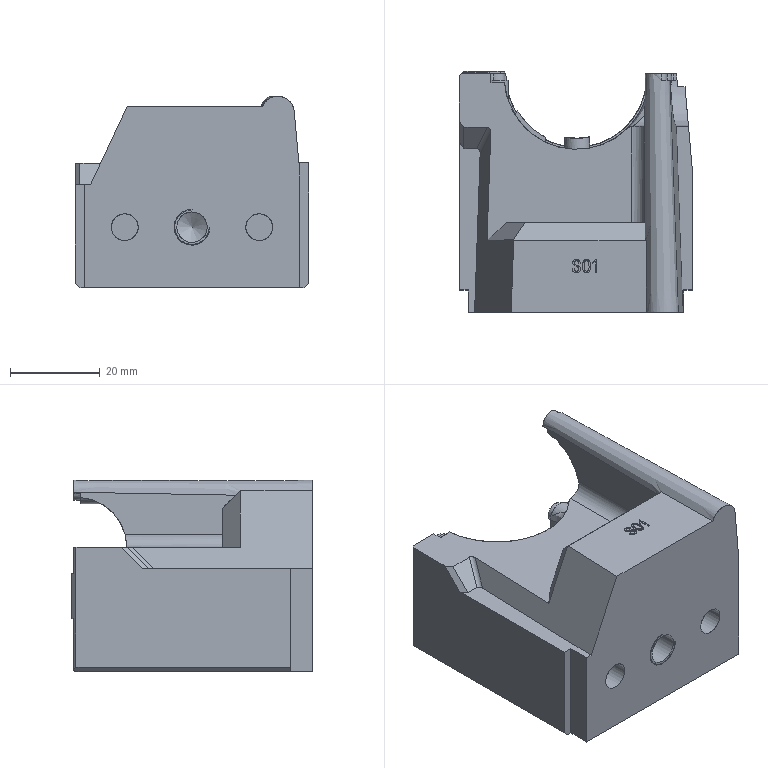NC program | PowerMill | posted with a generic post | part box 52 x 53.756 x 42.711 mm
Whole program:
%
O0001
N104 ( POWERMILL CB  : 2026004.0)
N105 ( POST VER      : 2026.0.0.5161)
N106 ( OPTION FILE   : FANUC)
N107 ( OUTPUT WORKPLANE : 2)
N108 (  )
N109 ( TOOL LIST )
N110 (--------------------------------)
N111 ( NO. | ID | DIA.| TIP RAD|LENGTH)
N112 (--------------------------------)
N113 (    1|D6_3| 6.0 |  0.0   | 97.0 )
N114 (--------------------------------)
N115 (  )
N116 ( NUMBER OF TOOLPATHS: 3.0 )
N117 ( ESTIMATED PROGRAM DURATION: 0 HOURS 1 MIN 8 SEC)
N118 (  )
N119 G00 G21 G80 G40 G17
N120 G90
N121 G54
N122 G53 Z0.0
N123 (---------------)
N124 ( START TOOLPATH : 13精光-D6-偏置平坦面 )
N125 (---------------)
N126 ( TOOL NO.    :1 )
N127 ( TOOL TYPE   : ENDMILL)
N128 ( TOOL ID     : D6_3)
N129 ( TOOL DIA    : 6.0 LENGTH 97.0)
N130 T1
N131 M6
N132 S6500 M03
N133 G00 G90 X-26.4454 Y-5.7682
N134 G43 Z75.756 H1
N135
N136 G05 P10000 R8
N137 Z53.3774
N138 G01 Z50.3774 F300.0
N139 X-24.9141 Y-2.9983 F500.0
N140 X-24.0418
N141 G02 X-25.9642 Y-0.039 I1.3749 J2.9971
N142 G01 X-25.9644 Y17.0037
N143 G02 X-23.7195 Y20.1236 I3.2977 J-0.0052
N144 G03 X-23.4367 Y20.3989 I-0.1638 J0.4512
N145 G00 Z61.2534
N146 G01 X-10.731 Y12.6007 F10000.0
N147 G00 Z56.2534
N148 G01 Z53.2534 F300.0
N149 X-13.5107 Y11.0873 F500.0
N150 X-19.0121 Y8.875
N151 G03 X-20.1113 Y8.6617 I-0.529 J-0.2127
N152 G01 X-20.1065 Y3.6989
N153 G03 X-19.4315 Y2.9984 I0.7017 J0.0007
N154 G01 X-19.1967 Y2.9895
N155 G03 X-18.4719 Y3.7613 I0.0266 J0.7012
N156 G01 X-18.9738 Y8.7197
N157 G03 X-19.0121 Y8.875 I-0.5675 J-0.0575
N158 G01 X-16.4541 Y9.9037
N159 X-16.8444 Y10.9904
N160 G02 X-16.9453 Y13.5394 I3.9938 J1.4346
N161 G01 X-16.8778 Y13.7875
N162 G03 X-21.8546 Y15.5141 I-2.5473 J0.6934
N163 G01 X-22.6473 Y13.6501
N164 G03 X-22.8609 Y12.6126 I2.4645 J-1.0481
N165 G01 X-22.9066 Y1.0939
N166 G03 X-21.6715 Y-0.1103 I1.2 J-0.0048
N167 G01 X-16.9207 Y0.0287
N168 G03 X-15.8315 Y0.8088 I-0.0351 J1.1995
N169 G01 X-15.7415 Y1.0503
N170 G03 X-15.6658 Y1.4681 I-1.1243 J0.4193
N171 G01 X-15.6593 Y6.3917
N172 G03 X-16.0952 Y8.9046 I-7.4049 J0.0097
N173 G01 X-16.4541 Y9.9037
N174 X-13.5107 Y11.0873
N175 G00 Z61.3534
N176 G01 X18.689 Y1.1883 F10000.0
N177 G00 Z56.3534
N178 G01 Z53.3534 F300.0
N179 X18.7509 Y1.2416 Z53.352
N180 X19.0519 Y1.6035 Z53.3437
N181 X19.2892 Y2.01 Z53.3355
N182 X19.4564 Y2.45 Z53.3273
N183 X19.5489 Y2.9115 Z53.3191
N184 X19.5642 Y3.382 Z53.3109
N185 X19.5018 Y3.8485 Z53.3027
N186 X19.3635 Y4.2985 Z53.2945
N187 X19.153 Y4.7195 Z53.2862
N188 X18.8761 Y5.1001 Z53.278
N189 X18.5403 Y5.43 Z53.2698
N190 X18.1548 Y5.7001 Z53.2616
N191 X17.7301 Y5.9031 Z53.2534
N192 X16.7998 Y6.2566 F500.0
N193 G03 X15.4447 Y5.4189 I-0.3565 J-0.9382
N194 G01 X15.1452 Y2.4429
N195 G03 X17.4406 Y-0.0864 I2.2876 J-0.2302
N196 G01 X24.7973 Y-0.0614
N197 G03 X25.7715 Y0.847 I-0.0033 J0.9801
N198 G01 X26.0144 Y4.1563
N199 G03 X24.5856 Y5.4215 I-1.1968 J0.0879
N200 G01 X24.2381 Y5.3531
N201 G02 X17.7301 Y5.9031 I-2.2935 J11.6409
N202 G01 X18.7117 Y8.4862
N203 G02 X16.7657 Y10.2425 I1.03 J3.0976
N204 G03 X16.3946 Y10.5136 I-0.4342 J-0.2047
N205 G02 X13.9637 Y11.6713 I0.5149 J4.2123
N206 G03 X13.3385 Y11.7026 I-0.3308 J-0.3478
N207 G01 X13.2771 Y11.6576
N208 G00 Z61.2534
N209 G01 X32.0704 Y11.1193 F10000.0
N210 G00 Z56.2534
N211 G01 Z53.2534 F300.0
N212 X28.9054 Y11.1194 F500.0
N213 G03 X28.7048 Y10.8393 I0.264 J-0.4009
N214 G02 X25.504 Y8.3115 I-3.2085 J0.7725
N215 G01 X19.7159 Y8.3118
N216 G02 X18.7117 Y8.4862 I0.0413 J3.2157
N217 G01 X17.7301 Y5.9031
N218 G00 Z61.2534
N219 G01 X10.5783 Y20.2721 F10000.0
N220 G00 Z56.2534
N221 G01 Z53.2534 F300.0
N222 X13.2783 Y21.9236 F500.0
N223 X13.3362 Y21.8814
N224 G03 X13.9546 Y21.9074 I0.2937 J0.3796
N225 G02 X16.3416 Y23.0641 I2.9672 J-3.0822
N226 G03 X16.7191 Y23.3494 I-0.0631 J0.4758
N227 G02 X19.7159 Y25.3833 I3.0477 J-1.2658
N228 G01 X25.3232 Y25.3839
N229 G02 X26.4084 Y25.2552 I0.1387 J-3.47
N230 G02 X28.7225 Y22.7727 I-0.9016 J-3.1604
N231 G03 X28.9055 Y22.4776 I0.4719 J0.0882
N232 G00 Z61.7556
N233 G01 X31.5683 Y16.7109 F10000.0
N234 G00 Z56.7556
N235 G01 Z53.7556 F300.0
N236 X28.4033 F500.0
N237 X22.6564 Y16.8153
N238 X22.6827 Y18.2647
N239 G03 X20.7553 Y19.2407 I-1.1998 J0.0218
N240 G01 X18.863 Y17.7977
N241 G03 X18.3916 Y16.8925 I0.7276 J-0.9542
N242 G01 X18.3882 Y16.8091
N243 G03 X18.8705 Y15.7976 I1.199 J-0.049
N244 G01 X20.7136 Y14.4251
N245 G03 X22.6301 Y15.3658 I0.7167 J0.9625
N246 G01 X22.6564 Y16.8153
N247 X25.5433 Y16.7629
N248 X25.581 Y21.0927
N249 G03 X25.0686 Y22.0576 I-1.1458 J0.01
N250 G01 X24.8221 Y22.2211
N251 G03 X24.1317 Y22.4208 I-0.6633 J-1.0
N252 G01 X20.3344 Y22.3351
N253 G03 X19.8645 Y22.1934 I0.0208 J-0.9186
N254 G01 X19.3635 Y21.8738
N255 X18.6194 Y21.2538
N256 G02 X17.5611 Y20.5217 I-4.4866 J5.3545
N257 G01 X16.5984 Y19.9795
N258 G03 X15.3082 Y17.7539 I1.2435 J-2.2076
N259 G01 X15.3226 Y15.728
N260 G03 X16.5496 Y13.6478 I2.4057 J0.017
N261 G01 X17.9604 Y12.8549
N262 G02 X18.8603 Y12.1949 I-2.269 J-4.0372
N263 G01 X19.0328 Y12.033
N264 G03 X19.3305 Y11.8283 I0.8211 J0.8751
N265 G01 X20.0888 Y11.4607
N266 G03 X20.952 Y11.2737 I0.817 J1.6856
N267 G01 X24.3418 Y11.3573
N268 G03 X25.1299 Y11.7806 I-0.0244 J0.9908
N269 G01 X25.2916 Y12.012
N270 G03 X25.5078 Y12.6887 I-0.9838 J0.6871
N271 G01 X25.5433 Y16.7629
N272 X28.4033 Y16.7109
N273 G00 Z61.2534
N274 G01 X-11.762 Y34.5911 F10000.0
N275 G00 Z56.2534
N276 G01 Z53.2534 F300.0
N277 X-14.1292 Y36.692 F500.0
N278 X-15.788 Y38.9844
N279 G03 X-15.382 Y39.4993 I-0.7035 J0.9722
N280 G01 X-15.1157 Y40.1455
N281 G03 X-15.6327 Y41.8289 I-1.2806 J0.5278
N282 G01 X-16.3655 Y42.3132
N283 G03 X-16.6494 Y42.4511 I-0.6615 J-1.0011
N284 G01 X-17.393 Y42.6976
N285 G03 X-20.4903 Y40.3123 I-0.7425 J-2.2393
N286 G03 X-17.1222 Y38.3277 I2.3548 J0.146
N287 G01 X-15.976 Y38.8729
N288 G03 X-15.788 Y38.9844 I-0.5155 J1.0837
N289 G01 X-14.1292 Y36.692
N290 G00 Z75.756
N291 G05 P0
N292 (---------------)
N293 ( END TOOLPATH : 13精光-D6-偏置平坦面 )
N294 (---------------)
N295 ( START TOOLPATH : 14精光-D6-等高 )
N296 (---------------)
N297 G00 X18.4844 Y24.8659 Z75.756
N298 G05 P10000 R8
N299 Z56.7076
N300 G01 Z53.7076 F1500.0
N301 G03 X19.1051 Y24.8414 I0.356 J1.1459 F2500.0
N302 G02 X19.7336 Y24.9151 I0.6618 J-2.9262
N303 G01 X25.1068 Y24.9146
N304 G02 X25.7022 Y24.8431 I-0.058 J-2.9959
N305 G03 X26.3229 Y24.8692 I0.2617 J1.1711
N306 G01 X26.3255 Y24.87
N307 X26.342 Y24.878 Z53.7012
N308 X26.3485 Y24.887 Z53.6853
N309 X26.3484 Y24.8882 Z53.6826
N310 X26.3405 Y24.8932 Z53.6651
N311 X26.3223 Y24.8905 Z53.6577
N312 G02 X25.7022 Y24.8538 I-0.3785 J1.1388
N313 G03 X25.1068 Y24.9153 I-0.6046 J-2.9424
N314 G01 X19.7336 Y24.9151
N315 G03 X19.1051 Y24.8414 I0.0333 J-2.9999
N316 G02 X18.4844 Y24.8659 I-0.2647 J1.1704
N317 G01 X18.4676 Y24.8711 Z53.6503
N318 X18.4606 Y24.8733 Z53.6327
N319 X18.4676 Y24.8711 Z53.615
N320 X18.4844 Y24.8659 Z53.6077
N321 G03 X19.1051 Y24.8414 I0.356 J1.1459
N322 G02 X19.7336 Y24.9151 I0.6618 J-2.9262
N323 G01 X25.1068 Y24.9153
N324 G02 X25.7022 Y24.8636 I0.0362 J-3.0408
N325 G03 X26.3216 Y24.9113 I0.2207 J1.1796
N326 G01 X26.324 Y24.9122
N327 X26.3401 Y24.9204 Z53.6012
N328 X26.3463 Y24.9289 Z53.5852
N329 Y24.9299 Z53.5826
N330 X26.3384 Y24.9339 Z53.5652
N331 X26.3207 Y24.9303 Z53.5577
N332 G02 X25.7022 Y24.8726 I-0.4168 J1.1252
N333 G03 X25.2482 Y24.9149 I-0.5046 J-2.9612
N334 G01 X19.7336 Y24.9151
N335 G03 X19.1051 Y24.8414 I0.0333 J-2.9999
N336 G02 X18.4844 Y24.8658 I-0.2647 J1.1704
N337 G01 X18.4676 Y24.8711 Z53.5504
N338 X18.4606 Y24.8733 Z53.5328
N339 X18.4676 Y24.8711 Z53.5151
N340 X18.4844 Y24.8659 Z53.5078
N341 G03 X19.1051 Y24.8414 I0.356 J1.1459
N342 G02 X19.7336 Y24.9151 I0.6618 J-2.9259
N343 G01 X25.2482 Y24.9153
N344 G02 X25.7022 Y24.8807 I-0.0007 J-3.0043
N345 G03 X26.3197 Y24.9488 I0.1817 J1.1862
N346 G01 X26.3221 Y24.9497
N347 X26.3378 Y24.9584 Z53.5013
N348 X26.3438 Y24.9669 Z53.4853
N349 X26.3437 Y24.9678 Z53.4827
N350 X26.3358 Y24.9713 Z53.4653
N351 X26.3184 Y24.967 Z53.4578
N352 G02 X25.7022 Y24.8879 I-0.4557 J1.1102
N353 G03 X25.2482 Y24.9153 I-0.4121 J-3.0551
N354 G01 X19.7336 Y24.9151
N355 G03 X19.1051 Y24.8414 I0.0333 J-2.9999
N356 G02 X18.4844 Y24.8659 I-0.2647 J1.1704
N357 G01 X18.4836 Y24.8661
N358 X18.4672 Y24.872 Z53.4508
N359 X18.4604 Y24.876 Z53.4337
N360 Y24.8761 Z53.4328
N361 X18.4675 Y24.8759 Z53.4152
N362 X18.4844 Y24.8714 Z53.4079
N363 G03 X19.1051 Y24.847 I0.356 J1.146
N364 G02 X19.7336 Y24.9207 I0.6618 J-2.9261
N365 G01 X25.3896 Y24.9206
N366 G02 X25.7022 Y24.8998 I-0.0423 J-3.0009
N367 G03 X26.3171 Y24.9885 I0.142 J1.1916
N368 G01 X26.3222 Y24.9907
N369 X26.3383 Y25.0017 Z53.4021
N370 X26.3443 Y25.0147 Z53.3875
N371 X26.3441 Y25.018 Z53.3828
N372 X26.335 Y25.0263 Z53.3655
N373 X26.3155 Y25.023 Z53.3579
N374 G02 X25.7022 Y24.9243 I-0.4909 J1.095
N375 G03 X25.3896 Y24.9399 I-0.3053 J-2.9786
N376 G01 X19.7336 Y24.9398
N377 G03 X19.105 Y24.866 I0.0332 J-2.9998
N378 G02 X18.4843 Y24.8905 I-0.2647 J1.1705
N379 G01 X18.4792 Y24.892
N380 X18.4613 Y24.9021 Z53.352
N381 X18.4542 Y24.9158 Z53.3371
N382 X18.4541 Y24.919 Z53.3329
N383 X18.4633 Y24.9295 Z53.3156
N384 X18.4842 Y24.9289 Z53.3079
N385 G03 X19.1048 Y24.9045 I0.3558 J1.146
N386 G02 X19.7336 Y24.9783 I0.662 J-2.9259
N387 G01 X25.3896 Y24.9785
N388 G02 X25.7015 Y24.9676 I0.0413 J-3.278
N389 G03 X26.3128 Y25.0783 I0.0991 J1.1959
N390 G01 X26.332 Y25.0873
N391 X26.362 Y25.1136 Z53.3033
N392 X26.3721 Y25.1506 Z53.2911
N393 X26.3711 Y25.1726 Z53.2825
N394 X26.3615 Y25.1963 Z53.2716
N395 X26.3353 Y25.2095 Z53.2614
N396 X26.3082 Y25.2042 Z53.258
N397 G02 X25.7022 Y25.0677 I-0.5578 J1.0625
N398 G01 X25.531 Y25.0745
N399 X19.7336
N400 G03 X19.1044 Y25.0007 I0.0331 J-2.9998
N401 G02 X18.4838 Y25.025 I-0.2649 J1.1704
N402 G00 Z58.791
N403 G01 X18.5529 Y8.8772 F10000.0
N404 G00 Z56.7076
N405 G01 Z53.7076 F1500.0
N406 G02 X19.1729 Y8.9159 I0.3824 J-1.1375 F2500.0
N407 G03 X19.7336 Y8.8567 I0.594 J2.9408
N408 G01 X25.1068 Y8.8571
N409 G03 X25.7026 Y8.9288 I-0.0594 J3.0046
N410 G02 X26.3232 Y8.9027 I0.2616 J-1.1711
N411 G01 X26.3277 Y8.9013
N412 X26.3452 Y8.8916 Z53.7017
N413 X26.352 Y8.8789 Z53.6866
N414 Y8.8761 Z53.6825
N415 X26.3431 Y8.8668 Z53.6652
N416 X26.323 Y8.8682 Z53.6577
N417 G03 X25.7029 Y8.9048 I-0.3783 J-1.1388
N418 G02 X25.1068 Y8.8432 I-0.6052 J2.9416
N419 G01 X19.7336 Y8.8433
N420 G02 X19.1729 Y8.9025 I0.0334 J3.0001
N421 G03 X18.553 Y8.8638 I-0.2376 J-1.1762
N422 G01 X18.5511 Y8.8631
N423 X18.535 Y8.8559 Z53.651
N424 X18.5285 Y8.8493 Z53.6346
N425 Y8.8488 Z53.6327
N426 X18.5358 Y8.8465 Z53.6151
N427 X18.553 Y8.8503 Z53.6077
N428 G02 X19.173 Y8.8891 I0.3824 J-1.1374
N429 G03 X19.7336 Y8.8299 I0.5939 J2.9408
N430 G01 X25.1068 Y8.8298
N431 G03 X25.703 Y8.8816 I0.0361 J3.0416
N432 G02 X26.3224 Y8.834 I0.221 J-1.1795
N433 G01 X26.3267 Y8.8325
N434 X26.3436 Y8.8226 Z53.6017
N435 X26.35 Y8.8103 Z53.5867
N436 X26.3499 Y8.8077 Z53.5826
N437 X26.3411 Y8.7995 Z53.5653
N438 X26.3215 Y8.8017 Z53.5577
N439 G03 X25.703 Y8.8592 I-0.4166 J-1.1254
N440 G02 X25.2482 Y8.8168 I-0.505 J2.9584
N441 G01 X19.7336 Y8.8166
N442 G02 X19.173 Y8.8758 I0.0334 J2.9999
N443 G03 X18.5531 Y8.837 I-0.2375 J-1.1763
N444 G01 X18.5512 Y8.8363
N445 X18.5351 Y8.8291 Z53.5511
N446 X18.5286 Y8.8225 Z53.5347
N447 Y8.822 Z53.5328
N448 X18.5359 Y8.8197 Z53.5152
N449 X18.5532 Y8.8235 Z53.5078
N450 G02 X19.1731 Y8.8623 I0.3824 J-1.1374
N451 G03 X19.7336 Y8.8032 I0.5938 J2.9407
N452 G01 X25.2482 Y8.803
N453 G03 X25.7028 Y8.8377 I0.0002 J2.9965
N454 G02 X26.3203 Y8.7698 I0.182 J-1.1861
N455 G01 X26.3246 Y8.7681
N456 X26.341 Y8.7578 Z53.5018
N457 X26.3471 Y8.7455 Z53.4868
N458 X26.3469 Y8.7429 Z53.4827
N459 X26.3379 Y8.7351 Z53.4654
N460 X26.3186 Y8.7381 Z53.4578
N461 G03 X25.7025 Y8.817 I-0.4554 J-1.1103
N462 G02 X25.2482 Y8.7896 I-0.4117 J3.0468
N463 G01 X19.7336 Y8.7898
N464 G02 X19.1732 Y8.8489 I0.0333 J2.9999
N465 G03 X18.5532 Y8.8101 I-0.2375 J-1.1762
N466 G01 X18.5513 Y8.8095
N467 X18.5352 Y8.8023 Z53.4512
N468 X18.5287 Y8.7957 Z53.4348
N469 Y8.7951 Z53.4328
N470 X18.536 Y8.7929 Z53.4153
N471 X18.5533 Y8.7967 Z53.4079
N472 G02 X19.1732 Y8.8355 I0.3825 J-1.1374
N473 G03 X19.7336 Y8.7764 I0.5937 J2.9408
N474 G01 X25.3896 Y8.7765
N475 G03 X25.7014 Y8.7971 I-0.0419 J3.0042
N476 G02 X26.3162 Y8.7081 I0.1413 J-1.1916
N477 G01 X26.3211 Y8.706
N478 X26.3375 Y8.6947 Z53.4021
N479 X26.3433 Y8.6813 Z53.3874
N480 X26.343 Y8.678 Z53.3828
N481 X26.3335 Y8.6694 Z53.3655
N482 X26.3138 Y8.6726 Z53.3579
N483 G03 X25.7006 Y8.7721 I-0.4923 J-1.0944
N484 G02 X25.3896 Y8.7568 I-0.3038 J3.0
N485 G01 X19.7336 Y8.757
N486 G02 X19.1733 Y8.8161 I0.0333 J2.9997
N487 G03 X18.5534 Y8.7772 I-0.2374 J-1.1763
N488 G01 X18.548 Y8.7754
N489 X18.5304 Y8.765 Z53.3521
N490 X18.5235 Y8.7512 Z53.3373
N491 Y8.7478 Z53.3329
N492 X18.5327 Y8.7375 Z53.3156
N493 X18.5535 Y8.7385 Z53.3079
N494 G02 X19.1735 Y8.7775 I0.3826 J-1.1373
N495 G03 X19.7336 Y8.7184 I0.5933 J2.9407
N496 G01 X25.3896 Y8.7182
N497 G03 X25.701 Y8.729 I0.0434 J3.2543
N498 G02 X26.3122 Y8.6182 I0.0988 J-1.196
N499 G01 X26.3315 Y8.609
N500 X26.3614 Y8.5829 Z53.3033
N501 X26.3715 Y8.5463 Z53.2911
N502 X26.3706 Y8.5241 Z53.2825
N503 X26.3612 Y8.5006 Z53.2716
N504 X26.3351 Y8.4874 Z53.2614
N505 X26.3082 Y8.4926 Z53.258
N506 G03 X25.7022 Y8.629 I-0.5575 J-1.0626
N507 G01 X25.531 Y8.6221
N508 X19.7336 Y8.6222
N509 G02 X19.1739 Y8.6811 I0.0332 J2.9997
N510 G03 X18.5539 Y8.6421 I-0.2372 J-1.1763
N511 G00 Z75.756
N512 G05 P0
N513 (---------------)
N514 ( END TOOLPATH : 14精光-D6-等高 )
N515 (---------------)
N516 ( START TOOLPATH : 26精光-D6-等高 )
N517 (---------------)
N518 G00 X-25.5772 Y-1.0586 Z75.756
N519 G05 P10000 R8
N520 Z56.208
N521 G01 Z53.208 F1500.0
N522 G03 X-25.4164 Y-0.4586 I-1.0392 J0.5999 F2500.0
N523 G01 X-25.4165 Y0.1414
N524 X-25.4171 Y13.5592
N525 Y14.1592
N526 G03 X-25.5779 Y14.7592 I-1.2 J-0.0001
N527 G01 X-25.5803 Y14.7633
N528 X-25.5882 Y14.7773 Z53.2023
N529 X-25.5924 Y14.7851 Z53.1877
N530 X-25.5928 Y14.786 Z53.183
N531 X-25.5904 Y14.7825 Z53.1657
N532 X-25.5822 Y14.7686 Z53.1581
N533 G02 X-25.4214 Y14.1686 I-1.0392 J-0.6
N534 G01 Y13.5686
N535 Y0.1407
N536 Y-0.4593
N537 G02 X-25.5822 Y-1.0593 I-1.2 J0.0
N538 G01 X-25.5828 Y-1.0604
N539 X-25.5919 Y-1.0751 Z53.1512
N540 X-25.5968 Y-1.0813 Z53.1344
N541 X-25.5969 Z53.1331
N542 X-25.5948 Y-1.0751 Z53.1155
N543 X-25.5866 Y-1.0599 Z53.1081
N544 G03 X-25.4258 Y-0.4599 I-1.0392 J0.6
N545 G01 Y0.1401
N546 Y13.5781
N547 Y14.1781
N548 G03 X-25.5866 Y14.7781 I-1.2 J0.0
N549 G01 X-25.589 Y14.7822
N550 X-25.5969 Y14.7962 Z53.1024
N551 X-25.6011 Y14.804 Z53.0878
N552 X-25.6015 Y14.8049 Z53.0831
N553 X-25.5991 Y14.8014 Z53.0658
N554 X-25.591 Y14.7875 Z53.0581
N555 G02 X-25.4302 Y14.1875 I-1.0392 J-0.6
N556 G01 Y13.5875
N557 Y0.1395
N558 Y-0.4605
N559 G02 X-25.591 Y-1.0605 I-1.2 J0.0
N560 G01 X-25.5916 Y-1.0616
N561 X-25.6006 Y-1.0763 Z53.0513
N562 X-25.6056 Y-1.0825 Z53.0345
N563 X-25.6057 Z53.0331
N564 X-25.6035 Y-1.0763 Z53.0156
N565 X-25.5953 Y-1.0611 Z53.0082
N566 G03 X-25.4346 Y-0.4611 I-1.0393 J0.6
N567 G01 Y0.1389
N568 Y13.6004
N569 Y14.2004
N570 G03 X-25.5953 Y14.8004 I-1.2 J0.0
N571 G01 X-25.5989 Y14.8066
N572 X-25.6063 Y14.8202 Z53.0031
N573 X-25.6101 Y14.829 Z52.9899
N574 X-25.6107 Y14.8312 Z52.9832
N575 X-25.608 Y14.8295 Z52.9661
N576 X-25.5997 Y14.8164 Z52.9582
N577 G02 X-25.4389 Y14.2164 I-1.0392 J-0.6
N578 G01 Y13.6164
N579 Y0.1383
N580 Y-0.4617
N581 G02 X-25.5997 Y-1.0617 I-1.2 J0.0
N582 G01 X-25.6004 Y-1.0628
N583 X-25.6094 Y-1.0775 Z52.9514
N584 X-25.6143 Y-1.0837 Z52.9345
N585 X-25.6144 Z52.9332
N586 X-25.6122 Y-1.0775 Z52.9156
N587 X-25.6041 Y-1.0623 Z52.9082
N588 G03 X-25.4433 Y-0.4623 I-1.0392 J0.6
N589 G01 Y0.1377
N590 Y13.6324
N591 Y14.2324
N592 G03 X-25.6041 Y14.8324 I-1.2 J0.0
N593 G01 X-25.6076 Y14.8385
N594 X-25.615 Y14.8522 Z52.9032
N595 X-25.6188 Y14.861 Z52.89
N596 X-25.6194 Y14.8631 Z52.8833
N597 X-25.6168 Y14.8615 Z52.8661
N598 X-25.6084 Y14.8483 Z52.8583
N599 G02 X-25.4477 Y14.2483 I-1.0393 J-0.6
N600 G01 Y13.6483
N601 Y0.1371
N602 Y-0.4629
N603 G02 X-25.6084 Y-1.0629 I-1.2 J0.0
N604 G01 X-25.6091 Y-1.0641
N605 X-25.6181 Y-1.0787 Z52.8514
N606 X-25.623 Y-1.0849 Z52.8346
N607 X-25.6232 Z52.8333
N608 X-25.621 Y-1.0787 Z52.8157
N609 X-25.6128 Y-1.0635 Z52.8083
N610 G03 X-25.452 Y-0.4635 I-1.0392 J0.6
N611 G01 Y0.1365
N612 Y13.6643
N613 Y14.2643
N614 G03 X-25.6128 Y14.8643 I-1.2 J0.0
N615 G01 X-25.6164 Y14.8705
N616 X-25.6237 Y14.8841 Z52.8033
N617 X-25.6276 Y14.8929 Z52.7901
N618 X-25.6282 Y14.8951 Z52.7833
N619 X-25.6255 Y14.8934 Z52.7662
N620 X-25.6172 Y14.8803 Z52.7584
N621 G02 X-25.4564 Y14.2803 I-1.0392 J-0.6
N622 G01 Y13.6803
N623 Y0.1359
N624 Y-0.4641
N625 G02 X-25.6172 Y-1.0641 I-1.2 J0.0
N626 G01 X-25.6178 Y-1.0653
N627 X-25.6269 Y-1.08 Z52.7515
N628 X-25.6318 Y-1.0861 Z52.7347
N629 X-25.6319 Z52.7334
N630 X-25.6297 Y-1.0799 Z52.7158
N631 X-25.6215 Y-1.0647 Z52.7084
N632 G03 X-25.4608 Y-0.4647 I-1.0393 J0.6
N633 G01 Y0.1353
N634 Y13.6963
N635 Y14.2963
N636 G03 X-25.6215 Y14.8963 I-1.2 J0.0
N637 G01 X-25.6251 Y14.9024
N638 X-25.6325 Y14.9161 Z52.7034
N639 X-25.6363 Y14.9249 Z52.6902
N640 X-25.6369 Y14.9271 Z52.6834
N641 X-25.6343 Y14.9254 Z52.6663
N642 X-25.6259 Y14.9123 Z52.6584
N643 G02 X-25.4651 Y14.3123 I-1.0393 J-0.6
N644 G01 Y13.7123
N645 Y0.1347
N646 Y-0.4653
N647 G02 X-25.6259 Y-1.0653 I-1.2001 J0.0
N648 G01 X-25.6266 Y-1.0665
N649 X-25.6356 Y-1.0812 Z52.6516
N650 X-25.6405 Y-1.0873 Z52.6348
N651 X-25.6406 Z52.6335
N652 X-25.6385 Y-1.0811 Z52.6159
N653 X-25.6303 Y-1.0659 Z52.6085
N654 G03 X-25.4695 Y-0.4659 I-1.0392 J0.6
N655 G01 Y0.1341
N656 Y13.7282
N657 Y14.3282
N658 G03 X-25.6303 Y14.9282 I-1.2 J0.0
N659 G01 X-25.6338 Y14.9342
N660 X-25.6411 Y14.948 Z52.6034
N661 X-25.6447 Y14.9569 Z52.5901
N662 X-25.6451 Y14.9591 Z52.5835
N663 X-25.6421 Y14.9574 Z52.5664
N664 X-25.6336 Y14.9443 Z52.5585
N665 G02 X-25.4733 Y14.3442 I-1.0397 J-0.5992
N666 G01 X-25.4738 Y13.7442
N667 X-25.4739 Y13.592
N668 Y0.1335
N669 Y-0.4665
N670 G02 X-25.6347 Y-1.0665 I-1.2 J0.0
N671 G01 X-25.6353 Y-1.0677
N672 X-25.6444 Y-1.0824 Z52.5517
N673 X-25.6493 Y-1.0885 Z52.5349
N674 X-25.6494 Y-1.0886 Z52.5335
N675 X-25.6472 Y-1.0823 Z52.516
N676 X-25.639 Y-1.0671 Z52.5086
N677 G03 X-25.4783 Y-0.4671 I-1.0393 J0.6
N678 G01 Y0.1329
N679 Y13.592
N680 X-25.478 Y13.7602
N681 X-25.4769 Y14.3602
N682 G03 X-25.6367 Y14.9605 I-1.2 J0.0021
N683 G01 X-25.6401 Y14.9664
N684 X-25.6474 Y14.9802 Z52.5035
N685 X-25.651 Y14.9892 Z52.4902
N686 X-25.6514 Y14.9913 Z52.4836
N687 X-25.6484 Y14.9897 Z52.4664
N688 X-25.6399 Y14.9765 Z52.4586
N689 G02 X-25.4807 Y14.3761 I-1.0408 J-0.5973
N690 G01 X-25.4822 Y13.7761
N691 X-25.4826 Y13.592
N692 Y0.1323
N693 Y-0.4677
N694 G02 X-25.6434 Y-1.0677 I-1.2001 J0.0
N695 G01 X-25.6441 Y-1.0689
N696 X-25.6531 Y-1.0836 Z52.4517
N697 X-25.658 Y-1.0897 Z52.4349
N698 X-25.6581 Y-1.0898 Z52.4336
N699 X-25.6559 Y-1.0835 Z52.416
N700 X-25.6478 Y-1.0683 Z52.4086
N701 G03 X-25.487 Y-0.4683 I-1.0392 J0.6
N702 G01 Y0.1317
N703 Y13.592
N704 X-25.4864 Y13.7921
N705 X-25.4844 Y14.3921
N706 G03 X-25.6433 Y14.9926 I-1.2001 J0.0038
N707 G01 X-25.6468 Y14.9987
N708 X-25.6541 Y15.0124 Z52.4036
N709 X-25.6577 Y15.0213 Z52.3903
N710 X-25.6581 Y15.0235 Z52.3837
N711 X-25.6552 Y15.0218 Z52.3665
N712 X-25.6468 Y15.0087 Z52.3587
N713 G02 X-25.4883 Y14.4081 I-1.0415 J-0.5961
N714 G01 X-25.4906 Y13.8081
N715 X-25.4914 Y13.592
N716 Y0.1311
N717 Y-0.4689
N718 G02 X-25.6521 Y-1.0689 I-1.2 J0.0
N719 G01 X-25.6528 Y-1.0701
N720 X-25.6618 Y-1.0848 Z52.3518
N721 X-25.6668 Y-1.091 Z52.335
N722 X-25.6669 Z52.3337
N723 X-25.6647 Y-1.0847 Z52.3161
N724 X-25.6565 Y-1.0696 Z52.3087
N725 G03 X-25.4957 Y-0.4696 I-1.0393 J0.6001
N726 G01 Y0.1304
N727 Y13.592
N728 X-25.4948 Y13.824
N729 X-25.4922 Y14.424
N730 G03 X-25.6504 Y15.0247 I-1.2 J0.0051
N731 G01 X-25.6539 Y15.0308
N732 X-25.6612 Y15.0445 Z52.3036
N733 X-25.6648 Y15.0534 Z52.2904
N734 X-25.6653 Y15.0556 Z52.2837
N735 X-25.6625 Y15.0539 Z52.2666
N736 X-25.6541 Y15.0408 Z52.2588
N737 G02 X-25.4962 Y14.44 I-1.042 J-0.5952
N738 G01 X-25.499 Y13.84
N739 X-25.5001 Y13.592
N740 Y0.1298
N741 Y-0.4702
N742 G02 X-25.6609 Y-1.0702 I-1.2 J0.0001
N743 G01 X-25.6615 Y-1.0713
N744 X-25.6706 Y-1.086 Z52.2519
N745 X-25.6755 Y-1.0922 Z52.2351
N746 X-25.6756 Z52.2338
N747 X-25.6734 Y-1.086 Z52.2162
N748 X-25.6653 Y-1.0708 Z52.2088
N749 G03 X-25.5045 Y-0.4708 I-1.0392 J0.6
N750 G01 Y0.1292
N751 Y13.592
N752 X-25.5032 Y13.856
N753 X-25.5001 Y14.456
N754 G03 X-25.6579 Y15.0568 I-1.2 J0.006
N755 G01 X-25.6613 Y15.0629
N756 X-25.6686 Y15.0766 Z52.2037
N757 X-25.6723 Y15.0855 Z52.1905
N758 X-25.6728 Y15.0876 Z52.1838
N759 X-25.67 Y15.0859 Z52.1667
N760 X-25.6617 Y15.0728 Z52.1588
N761 G02 X-25.5041 Y14.4719 I-1.0424 J-0.5944
N762 G01 X-25.5074 Y13.872
N763 X-25.5089 Y13.592
N764 Y0.1286
N765 Y-0.4714
N766 G02 X-25.6696 Y-1.0714 I-1.2 J0.0
N767 G01 X-25.6703 Y-1.0725
N768 X-25.6793 Y-1.0872 Z52.152
N769 X-25.6842 Y-1.0934 Z52.1352
N770 X-25.6844 Z52.1339
N771 X-25.6822 Y-1.0872 Z52.1163
N772 X-25.674 Y-1.072 Z52.1089
N773 G03 X-25.5132 Y-0.472 I-1.0392 J0.6
N774 G01 Y0.128
N775 Y13.7334
N776 X-25.5101 Y13.9033
N777 X-25.4991 Y14.5032
N778 G03 X-25.6488 Y15.1061 I-1.1998 J0.0221
N779 G01 X-25.6503 Y15.1088
N780 X-25.6562 Y15.1395 Z52.1023
N781 X-25.6421 Y15.1631 Z52.0862
N782 X-25.6387 Y15.1654 Z52.0834
N783 X-25.612 Y15.1678 Z52.0663
N784 X-25.5896 Y15.1464 Z52.0589
N785 G02 X-25.4709 Y14.5367 I-1.0784 J-0.5264
N786 G01 X-25.5125 Y13.9381
N787 G03 X-25.5176 Y13.7334 I2.2825 J-0.1588
N788 G01 Y0.1274
N789 Y-0.4726
N790 G02 X-25.6784 Y-1.0726 I-1.2 J0.0
N791 G01 X-25.679 Y-1.0737
N792 X-25.6881 Y-1.0884 Z52.0521
N793 X-25.693 Y-1.0946 Z52.0353
N794 X-25.6931 Z52.0339
N795 X-25.6909 Y-1.0884 Z52.0164
N796 X-25.6827 Y-1.0732 Z52.009
N797 G03 X-25.522 Y-0.4732 I-1.0393 J0.6
N798 G01 Y0.1268
N799 Y13.7334
N800 G02 X-25.515 Y13.9729 I2.6791 J0.0416
N801 G01 X-25.4707 Y14.5713
N802 G03 X-25.5867 Y15.1815 I-1.1967 J0.0886
N803 G01 X-25.5923 Y15.1932
N804 X-25.5978 Y15.2075 Z52.0051
N805 X-25.5994 Y15.2191 Z51.9946
N806 X-25.5991 Y15.2265 Z51.984
N807 X-25.5941 Y15.229 Z51.9673
N808 X-25.585 Y15.2165 Z51.959
N809 G02 X-25.4711 Y14.6059 I-1.0824 J-0.5179
N810 G01 X-25.5174 Y14.0077
N811 G03 X-25.5263 Y13.7334 I3.0568 J-0.2368
N812 G01 Y0.1262
N813 Y-0.4738
N814 G02 X-25.6871 Y-1.0738 I-1.2001 J0.0
N815 G01 X-25.6878 Y-1.0749
N816 X-25.6968 Y-1.0896 Z51.9521
N817 X-25.7017 Y-1.0958 Z51.9353
N818 X-25.7018 Z51.934
N819 X-25.6997 Y-1.0896 Z51.9164
N820 X-25.6915 Y-1.0744 Z51.909
N821 G03 X-25.5307 Y-0.4744 I-1.0392 J0.6
N822 G01 Y0.1256
N823 Y13.7334
N824 G02 X-25.4333 Y14.534 I2.9526 J0.047
N825 G01 X-25.2802 Y15.1141
N826 G03 X-25.2825 Y15.7353 I-1.1603 J0.3063
N827 G01 X-25.2964 Y15.7864
N828 X-25.2986 Y15.8335 Z51.9059
N829 X-25.2806 Y15.8764 Z51.897
N830 X-25.2478 Y15.9215 Z51.8835
N831 X-25.2208 Y15.9391 Z51.8737
N832 X-25.1843 Y15.9301 Z51.8627
N833 X-25.1667 Y15.9015 Z51.8591
N834 G02 X-25.2002 Y15.2813 I-1.1742 J-0.2476
N835 G01 X-25.3865 Y14.7109
N836 G03 X-25.5351 Y13.7334 I2.8636 J-0.9353
N837 G01 Y0.125
N838 Y-0.475
N839 G02 X-25.6959 Y-1.075 I-1.2 J0.0
N840 G01 X-25.6965 Y-1.0761
N841 X-25.7055 Y-1.0908 Z51.8522
N842 X-25.7105 Y-1.097 Z51.8354
N843 X-25.7106 Z51.8341
N844 X-25.7084 Y-1.0908 Z51.8165
N845 X-25.7002 Y-1.0756 Z51.8091
N846 G03 X-25.5395 Y-0.4756 I-1.0393 J0.6
N847 G01 Y0.1244
N848 Y13.7334
N849 G02 X-25.3627 Y14.7933 I3.015 J0.042
N850 G01 X-25.1602 Y15.3581
N851 G03 X-25.1089 Y15.9771 I-1.1295 J0.4051
N852 G01 X-25.1136 Y16.0028
N853 X-25.113 Y16.0287 Z51.8057
N854 X-25.1022 Y16.0505 Z51.7962
N855 X-25.0866 Y16.0691 Z51.7839
N856 X-25.0725 Y16.0765 Z51.7737
N857 X-25.055 Y16.0692 Z51.7628
N858 X-25.0471 Y16.0523 Z51.7592
N859 G02 X-25.1166 Y15.435 I-1.1866 J-0.1789
N860 G01 X-25.3358 Y14.8765
N861 G03 X-25.5438 Y13.7334 I2.8056 J-1.101
N862 G01 Y0.1243
N863 Y-0.4757
N864 G02 X-25.7046 Y-1.0757 I-1.2001 J0.0
N865 G01 X-25.7051 Y-1.0765
N866 X-25.7142 Y-1.0913 Z51.7522
N867 X-25.7192 Y-1.0973 Z51.7352
N868 X-25.7193 Z51.7342
N869 X-25.7172 Y-1.0908 Z51.7166
N870 X-25.709 Y-1.0755 Z51.7092
N871 G03 X-25.5482 Y-0.4755 I-1.0392 J0.6
N872 G01 Y0.1245
N873 Y16.5641
N874 Y17.1641
N875 G03 X-25.709 Y17.7641 I-1.2 J0.0
N876 G01 X-25.7206 Y17.7842
N877 X-25.727 Y17.7983 Z51.7065
N878 X-25.7298 Y17.8117 Z51.6987
N879 X-25.7311 Y17.8297 Z51.6842
N880 X-25.7253 Y17.8371 Z51.6682
N881 X-25.7133 Y17.8262 Z51.6592
N882 G02 X-25.5526 Y17.2262 I-1.0393 J-0.6
N883 G01 Y16.6262
N884 Y0.1247
N885 Y-0.4753
N886 G02 X-25.7133 Y-1.0753 I-1.2 J0.0
N887 G01 X-25.7138 Y-1.0761
N888 X-25.723 Y-1.0909 Z51.6523
N889 X-25.728 Y-1.0969 Z51.6352
N890 X-25.7281 Z51.6343
N891 X-25.7259 Y-1.0904 Z51.6166
N892 X-25.7177 Y-1.0751 Z51.6093
N893 G03 X-25.5569 Y-0.4751 I-1.0392 J0.6
N894 G01 Y0.1249
N895 Y16.6883
N896 Y17.2883
N897 G03 X-25.7177 Y17.8883 I-1.2 J0.0
N898 G01 X-25.7222 Y17.8962
N899 X-25.7293 Y17.9096 Z51.6047
N900 X-25.7328 Y17.9192 Z51.5926
N901 X-25.7335 Y17.9227 Z51.5843
N902 X-25.7306 Y17.9225 Z51.5673
N903 X-25.7221 Y17.9099 Z51.5593
N904 G02 X-25.5613 Y17.3099 I-1.0392 J-0.6
N905 G01 Y16.7099
N906 Y0.1251
N907 Y-0.4749
N908 G02 X-25.7221 Y-1.0749 I-1.2 J0.0
N909 G01 X-25.7226 Y-1.0758
N910 X-25.7317 Y-1.0906 Z51.5523
N911 X-25.7367 Y-1.0966 Z51.5353
N912 X-25.7368 Z51.5343
N913 X-25.7346 Y-1.0901 Z51.5167
N914 X-25.7265 Y-1.0748 Z51.5093
N915 G03 X-25.5657 Y-0.4748 I-1.0392 J0.6
N916 G01 Y0.1252
N917 Y16.7191
N918 Y17.3191
N919 G03 X-25.7265 Y17.9191 I-1.2 J0.0
N920 G01 X-25.7288 Y17.9231
N921 X-25.7368 Y17.9371 Z51.5036
N922 X-25.741 Y17.9449 Z51.4889
N923 X-25.7414 Y17.9457 Z51.4844
N924 X-25.739 Y17.9422 Z51.467
N925 X-25.7308 Y17.9282 Z51.4594
N926 G02 X-25.5701 Y17.3282 I-1.0393 J-0.6
N927 G01 Y16.7282
N928 Y0.1253
N929 Y-0.4747
N930 G02 X-25.7308 Y-1.0747 I-1.2 J0.0
N931 G01 X-25.7313 Y-1.0755
N932 X-25.7405 Y-1.0903 Z51.4524
N933 X-25.7455 Y-1.0963 Z51.4354
N934 Z51.4344
N935 X-25.7434 Y-1.0898 Z51.4168
N936 X-25.7352 Y-1.0745 Z51.4094
N937 G03 X-25.5744 Y-0.4745 I-1.0392 J0.6
N938 G01 Y0.1255
N939 Y16.7374
N940 Y17.3374
N941 G03 X-25.7352 Y17.9374 I-1.2 J0.0
N942 G01 X-25.7375 Y17.9415
N943 X-25.7455 Y17.9555 Z51.4037
N944 X-25.7497 Y17.9633 Z51.389
N945 X-25.7501 Y17.9641 Z51.3845
N946 X-25.7477 Y17.9605 Z51.3671
N947 X-25.7396 Y17.9466 Z51.3595
N948 G02 X-25.5788 Y17.3466 I-1.0392 J-0.6
N949 G01 Y16.7466
N950 Y0.1256
N951 Y-0.4744
N952 G02 X-25.7396 Y-1.0744 I-1.2 J0.0
N953 G01 X-25.7401 Y-1.0753
N954 X-25.7492 Y-1.0901 Z51.3525
N955 X-25.7542 Y-1.0961 Z51.3355
N956 X-25.7543 Z51.3345
N957 X-25.7521 Y-1.0896 Z51.3169
N958 X-25.7439 Y-1.0743 Z51.3095
N959 G03 X-25.5832 Y-0.4743 I-1.0393 J0.6
N960 G01 Y0.1257
N961 Y16.7558
N962 Y17.3558
N963 G03 X-25.7439 Y17.9558 I-1.2 J0.0
N964 G01 X-25.7463 Y17.9598
N965 X-25.7542 Y17.9738 Z51.3038
N966 X-25.7585 Y17.9816 Z51.2891
N967 X-25.7589 Y17.9825 Z51.2845
N968 X-25.7565 Y17.9789 Z51.2672
N969 X-25.7483 Y17.965 Z51.2595
N970 G02 X-25.5875 Y17.365 I-1.0392 J-0.6
N971 G01 Y16.765
N972 Y0.1258
N973 Y-0.4742
N974 G02 X-25.7483 Y-1.0742 I-1.2 J0.0
N975 G01 X-25.7488 Y-1.0751
N976 X-25.758 Y-1.0899 Z51.2526
N977 X-25.7629 Y-1.0959 Z51.2356
N978 X-25.763 Z51.2346
N979 X-25.7609 Y-1.0894 Z51.217
N980 X-25.7527 Y-1.0741 Z51.2096
N981 G03 X-25.5919 Y-0.4741 I-1.0392 J0.6
N982 G01 Y0.1259
N983 Y16.7742
N984 Y17.3742
N985 G03 X-25.7527 Y17.9742 I-1.2 J0.0
N986 G01 X-25.755 Y17.9782
N987 X-25.763 Y17.9922 Z51.2038
N988 X-25.7672 Y18.0 Z51.1892
N989 X-25.7676 Y18.0008 Z51.1846
N990 X-25.7652 Y17.9973 Z51.1673
N991 X-25.757 Y17.9834 Z51.1596
N992 G02 X-25.5963 Y17.3834 I-1.0393 J-0.6001
N993 G01 Y16.7834
N994 Y0.1259
N995 Y-0.4741
N996 G02 X-25.757 Y-1.0741 I-1.2 J0.0
N997 G01 X-25.7576 Y-1.075
N998 X-25.7667 Y-1.0897 Z51.1527
N999 X-25.7717 Y-1.0958 Z51.1357
N1000 X-25.7718 Z51.1346
N1001 X-25.7696 Y-1.0893 Z51.117
N1002 X-25.7614 Y-1.074 Z51.1097
N1003 G03 X-25.6006 Y-0.474 I-1.0393 J0.6
N1004 G01 Y0.126
N1005 Y16.7925
N1006 Y17.3925
N1007 G03 X-25.7614 Y17.9925 I-1.2001 J0.0
N1008 G01 X-25.7637 Y17.9966
N1009 X-25.7717 Y18.0106 Z51.1039
N1010 X-25.7759 Y18.0184 Z51.0892
N1011 X-25.7763 Y18.0192 Z51.0847
N1012 X-25.774 Y18.0156 Z51.0674
N1013 X-25.7658 Y18.0017 Z51.0597
N1014 G02 X-25.605 Y17.4017 I-1.0393 J-0.6
N1015 G01 Y16.8017
N1016 Y0.126
N1017 Y-0.474
N1018 G02 X-25.7658 Y-1.074 I-1.2 J0.0
N1019 G01 X-25.7663 Y-1.0749
N1020 X-25.7755 Y-1.0897 Z51.0528
N1021 X-25.7804 Y-1.0957 Z51.0358
N1022 X-25.7805 Z51.0347
N1023 X-25.7783 Y-1.0893 Z51.0171
N1024 X-25.7702 Y-1.074 Z51.0097
N1025 G03 X-25.6094 Y-0.474 I-1.0392 J0.6
N1026 G01 Y0.126
N1027 Y16.8109
N1028 Y17.4109
N1029 G03 X-25.7702 Y18.0109 I-1.2 J0.0
N1030 G01 X-25.7725 Y18.0149
N1031 X-25.7805 Y18.029 Z51.004
N1032 X-25.7847 Y18.0367 Z50.9893
N1033 X-25.7851 Y18.0376 Z50.9848
N1034 X-25.7827 Y18.034 Z50.9674
N1035 X-25.7745 Y18.0201 Z50.9598
N1036 G02 X-25.6138 Y17.4201 I-1.0393 J-0.6
N1037 G01 Y16.8201
N1038 Y0.126
N1039 Y-0.474
N1040 G02 X-25.7745 Y-1.074 I-1.2 J0.0001
N1041 G01 X-25.7751 Y-1.0749
N1042 X-25.7842 Y-1.0896 Z50.9528
N1043 X-25.7892 Y-1.0957 Z50.9359
N1044 X-25.7893 Z50.9348
N1045 X-25.7871 Y-1.0893 Z50.9172
N1046 X-25.7789 Y-1.074 Z50.9098
N1047 G03 X-25.6181 Y-0.474 I-1.0392 J0.6
N1048 G01 Y0.126
N1049 Y16.8293
N1050 Y17.4293
N1051 G03 X-25.7789 Y18.0293 I-1.2 J0.0
N1052 G01 X-25.7812 Y18.0333
N1053 X-25.7892 Y18.0473 Z50.9041
N1054 X-25.7934 Y18.0551 Z50.8894
N1055 X-25.7938 Y18.0559 Z50.8848
N1056 X-25.7914 Y18.0524 Z50.8675
N1057 X-25.7833 Y18.0385 Z50.8599
N1058 G02 X-25.6225 Y17.4385 I-1.0392 J-0.6
N1059 G01 Y16.8385
N1060 Y0.126
N1061 Y-0.474
N1062 G02 X-25.7833 Y-1.074 I-1.2 J0.0
N1063 G01 X-25.7838 Y-1.0749
N1064 X-25.7929 Y-1.0897 Z50.8529
N1065 X-25.7979 Y-1.0957 Z50.836
N1066 X-25.798 Z50.8349
N1067 X-25.7958 Y-1.0893 Z50.8173
N1068 X-25.7876 Y-1.074 Z50.8099
N1069 G03 X-25.6269 Y-0.474 I-1.0393 J0.6
N1070 G01 Y0.126
N1071 Y16.8454
N1072 Y17.4454
N1073 G03 X-25.7876 Y18.0454 I-1.2 J0.0
N1074 G01 X-25.7888 Y18.0475
N1075 X-25.7975 Y18.062 Z50.8034
N1076 X-25.8022 Y18.0687 Z50.7873
N1077 X-25.8024 Y18.0688 Z50.7849
N1078 X-25.8002 Y18.0635 Z50.7674
N1079 X-25.792 Y18.0487 Z50.7599
N1080 G02 X-25.6312 Y17.4487 I-1.0393 J-0.6
N1081 G01 Y16.8487
N1082 Y0.1259
N1083 Y-0.4741
N1084 G02 X-25.792 Y-1.0741 I-1.2001 J0.0
N1085 G01 X-25.7926 Y-1.075
N1086 X-25.8017 Y-1.0898 Z50.753
N1087 X-25.8066 Y-1.0958 Z50.7361
N1088 X-25.8067 Z50.735
N1089 X-25.8046 Y-1.0895 Z50.7174
N1090 X-25.7964 Y-1.0742 Z50.71
N1091 G03 X-25.6356 Y-0.4742 I-1.0392 J0.6
N1092 G01 Y0.1258
N1093 Y16.8521
N1094 Y17.4521
N1095 G03 X-25.7964 Y18.0521 I-1.2 J0.0
N1096 G01 X-25.7976 Y18.0542
N1097 X-25.8063 Y18.0686 Z50.7035
N1098 X-25.8109 Y18.0754 Z50.6874
N1099 X-25.8111 Y18.0755 Z50.685
N1100 X-25.8089 Y18.0702 Z50.6675
N1101 X-25.8008 Y18.0555 Z50.66
N1102 G02 X-25.64 Y17.4555 I-1.0392 J-0.6
N1103 G01 Y16.8555
N1104 Y0.1257
N1105 Y-0.4743
N1106 G02 X-25.8008 Y-1.0743 I-1.2 J0.0
N1107 G01 X-25.8013 Y-1.0753
N1108 X-25.8104 Y-1.09 Z50.6531
N1109 X-25.8154 Y-1.0961 Z50.6362
N1110 X-25.8155 Z50.635
N1111 X-25.8133 Y-1.0897 Z50.6175
N1112 X-25.8051 Y-1.0744 Z50.6101
N1113 G03 X-25.6444 Y-0.4744 I-1.0393 J0.6
N1114 G01 Y0.1256
N1115 Y16.859
N1116 Y17.459
N1117 G03 X-25.8051 Y18.059 I-1.2 J0.0
N1118 G01 X-25.8064 Y18.0611
N1119 X-25.815 Y18.0756 Z50.6036
N1120 X-25.8197 Y18.0823 Z50.5876
N1121 X-25.8199 Y18.0825 Z50.5851
N1122 X-25.8176 Y18.0772 Z50.5676
N1123 X-25.8095 Y18.0625 Z50.5601
N1124 G02 X-25.6487 Y17.4625 I-1.0392 J-0.6
N1125 G01 Y16.8625
N1126 Y0.1254
N1127 Y-0.4746
N1128 G02 X-25.8095 Y-1.0746 I-1.2 J0.0
N1129 G01 X-25.8101 Y-1.0756
N1130 X-25.8192 Y-1.0903 Z50.5532
N1131 X-25.8241 Y-1.0964 Z50.5363
N1132 X-25.8242 Z50.5351
N1133 X-25.8221 Y-1.09 Z50.5175
N1134 X-25.8139 Y-1.0747 Z50.5101
N1135 G03 X-25.6531 Y-0.4747 I-1.0392 J0.6
N1136 G01 Y0.1253
N1137 Y16.8662
N1138 Y17.4662
N1139 G03 X-25.8139 Y18.0662 I-1.2 J0.0
N1140 G01 X-25.8152 Y18.0684
N1141 X-25.8238 Y18.0828 Z50.5037
N1142 X-25.8284 Y18.0896 Z50.4877
N1143 X-25.8286 Y18.0898 Z50.4852
N1144 X-25.8264 Y18.0846 Z50.4677
N1145 X-25.8182 Y18.0699 Z50.4602
N1146 G02 X-25.6575 Y17.4699 I-1.0393 J-0.6
N1147 G01 Y16.8699
N1148 Y0.125
N1149 Y-0.475
N1150 G02 X-25.8182 Y-1.075 I-1.2 J0.0001
N1151 G01 X-25.8188 Y-1.076
N1152 X-25.8279 Y-1.0907 Z50.4533
N1153 X-25.8329 Y-1.0968 Z50.4364
N1154 X-25.833 Z50.4352
N1155 X-25.8308 Y-1.0905 Z50.4176
N1156 X-25.8226 Y-1.0752 Z50.4102
N1157 G03 X-25.6618 Y-0.4752 I-1.0393 J0.6
N1158 G01 Y0.1248
N1159 Y16.8738
N1160 Y17.4738
N1161 G03 X-25.8226 Y18.0738 I-1.2001 J0.0
N1162 G00 Z75.756
N1163 G05 P0
N1164 (---------------)
N1165 ( END TOOLPATH : 26精光-D6-等高 )
N1166 (---------------)
N1167
N1168 M05
N1169 G53 Z0.0
N1170 M30
%